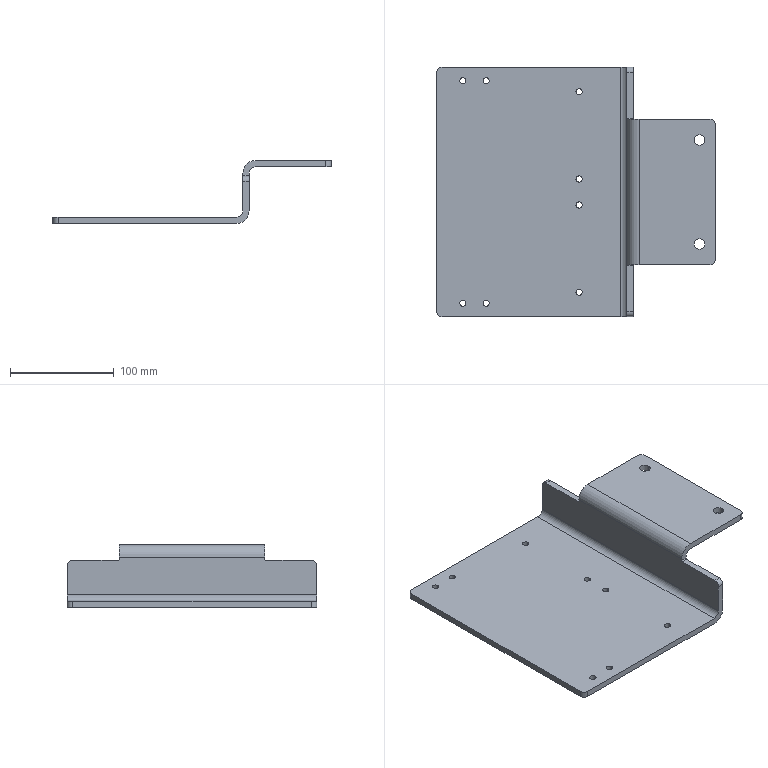Part | STEP file | [01]-10 | 1 solid | 46 faces | box 268 x 240 x 60.3 mm | volume 396415 mm3 | cylinder 32 | plane 14 | commonest cylinder face diameters 6 x16 10 x10 2 x2 12 x2 24 x2